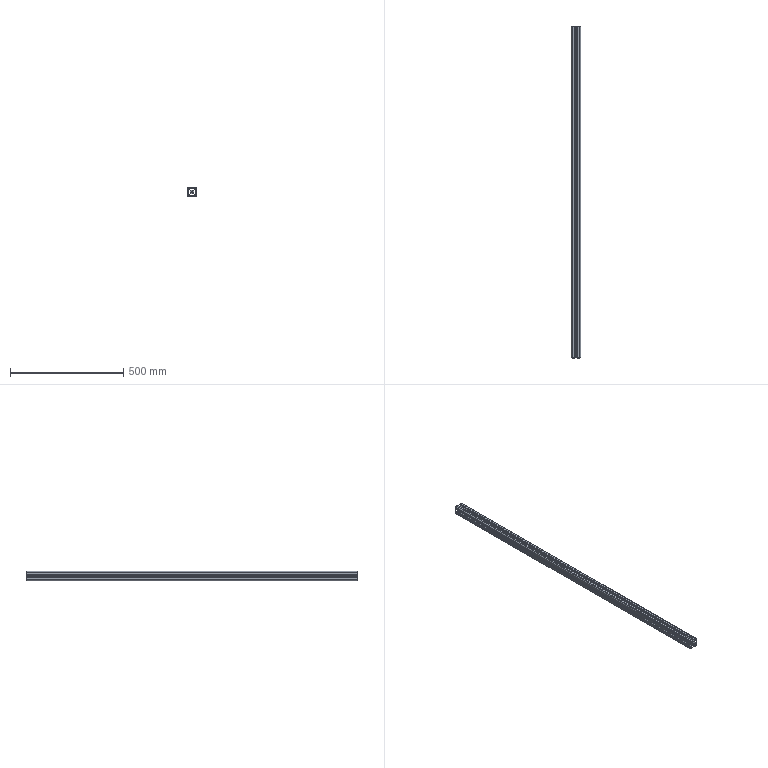Part | SolidWorks | features WeldMemberFeat 1, WeldmentFeature 1 | 1 solid | 92 faces | box 40 x 1467 x 40 mm | volume 887305 mm3 | plane 78 | cylinder 14 | commonest cylinder face diameters 6 x8 9 x4 6.8 x2